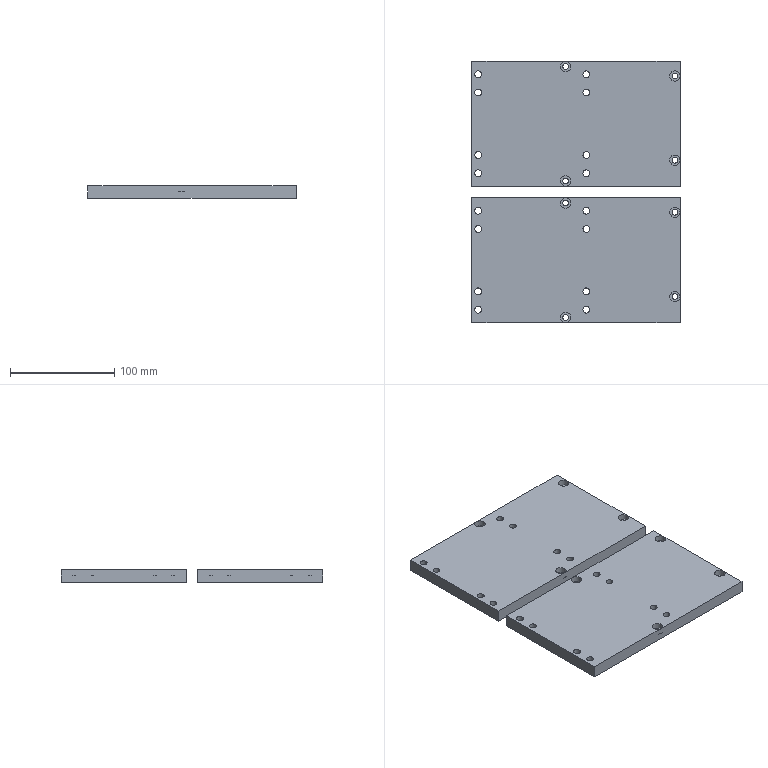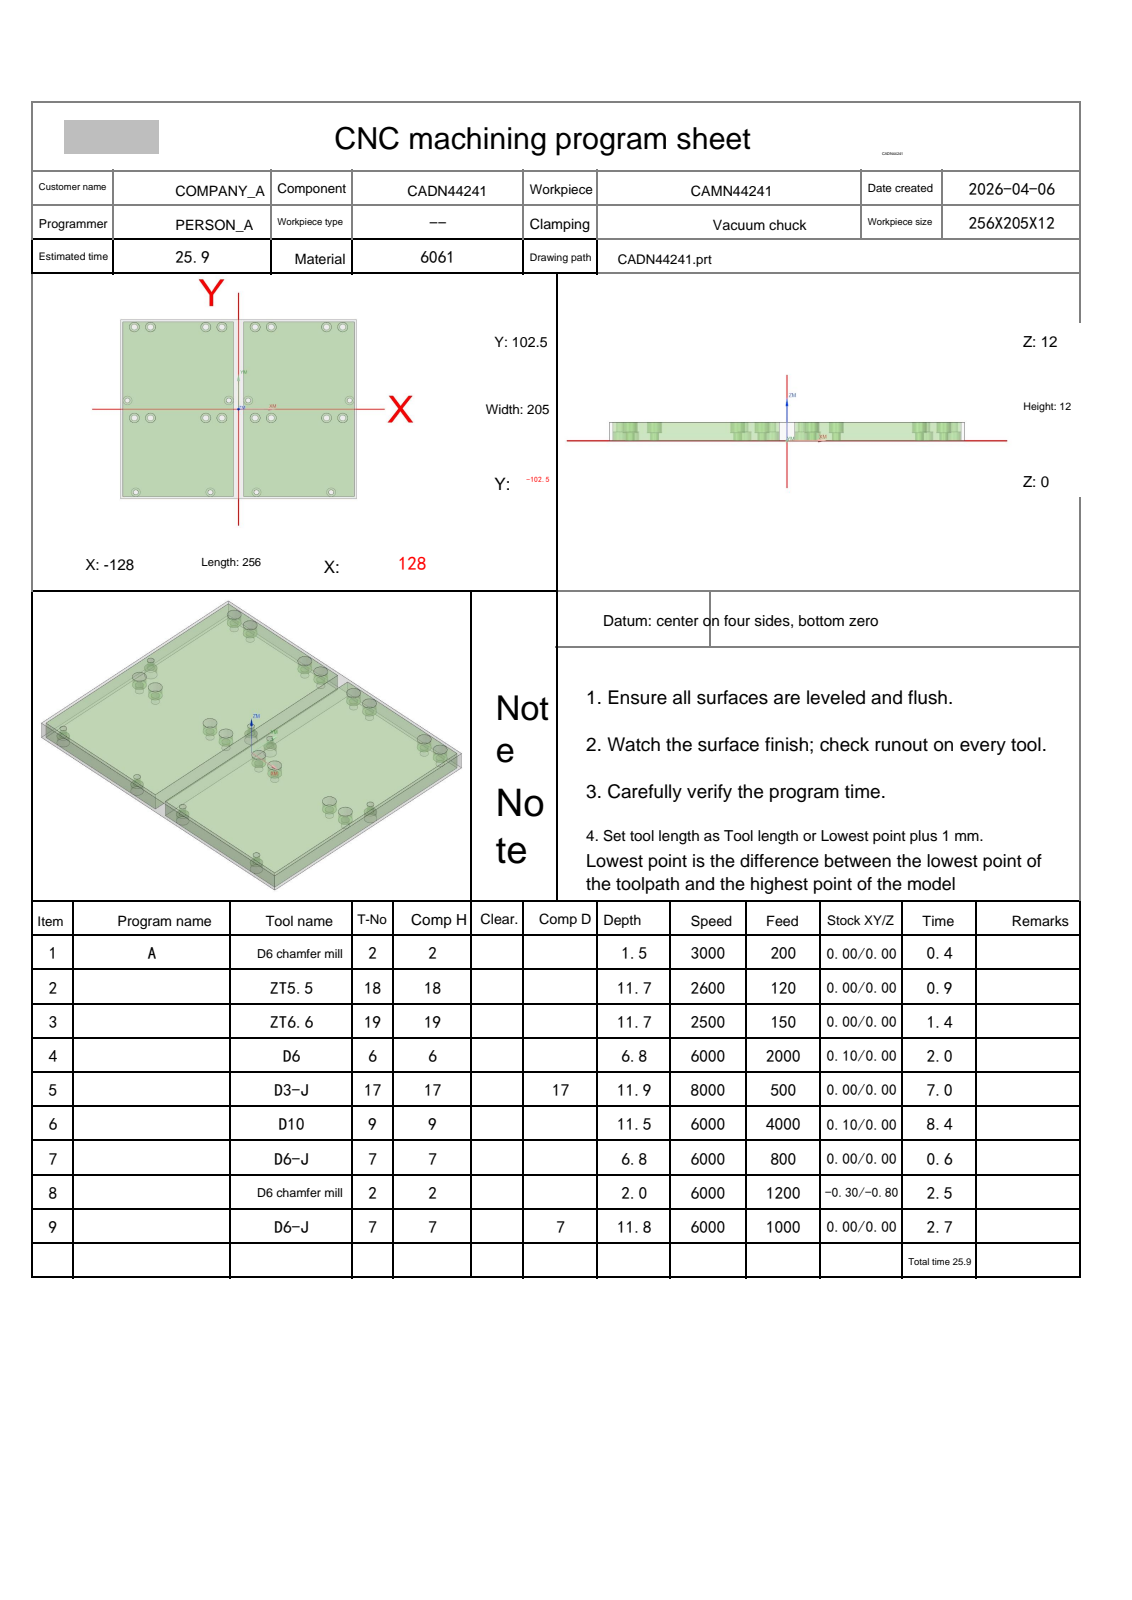NC program | NX | posted by the shop | part box 200 x 251 x 12 mm
Lines 1 to 557 of 3499:
%
O0001
(Machine time: 27.62 MIN)
(===Total Tool:7===)
(T2=D6 chamfer mill   D=6.   R=0.   D-  H02 Z=10.   )
(T18=ZT5.5  D=5.5  DR_a=118 D-  H18 Z=0.3   )
(T19=ZT6.6  D=6.6  DR_a=118 D-  H19 Z=0.3   )
(T6=D6      D=6.   R=0.   D-  H06 Z=5.2   )
(T17=D3-J   D=3.   R=0.   D17 H17 Z=0.15  )
(T9=D10     D=10.  R=0.   D-  H09 Z=0.5   )
(T7=D6-J    D=6.   R=0.   D-  H07 Z=0.2   )
G80 G90 G17 G49 G40
G91 G28 Z0
M01
N1 T02 M06
(D6 chamfer mill  D=6. R=0. H=02 ce=0.00 di=0.00)
G00 G90 G54 X100.5 Y-95. M03 S3000
G43 H02 Z32.
M08
G98 G81 X100.5 Y-95. Z10.5 R13. F200.
X19.5
X-30.5
X-111.5
X-113. Y-10.
X-120.5 Y10.
X-95.5 Y-10.
X-35.5
X-18.
X-10.5 Y10.
X10.5
X18. Y-10.
X35.5
X95.5
X113.
X120.5 Y10.
X113. Y94.
X95.5
X35.5
X18.
X-18.
X-35.5
X-95.5
X-113.
G80
G00 Z32.
G91 G28 Z0.0
M05
M09
G91 G28 Z0.0
M01
N2 T18 M06
(ZT5.5 D=5.5 DR_a=118 H=18)
G00 G90 G54 X10.5 Y10. M03 S2600
G43 H18 Z32.
M08
G98 G83 X10.5 Y10. Z.3 R13. F120. Q1.5
X-10.5
X-120.5
X-111.5 Y-95.
X-30.5
X19.5
X100.5
X120.5 Y10.
G80
G00 Z32.
G91 G28 Z0.0
M05
M09
G91 G28 Z0.0
M01
N3 T19 M06
(ZT6.6 D=6.6 DR_a=118 H=19)
G00 G90 G54 X-113. Y94. M03 S2500
G43 H19 Z32.
M08
G98 G83 X-113. Y94. Z.3 R13. F150. Q3.
X-95.5
X-35.5
X-18.
X18.
X35.5
X95.5
X113.
Y-10.
X95.5
X35.5
X18.
X-18.
X-35.5
X-95.5
X-113.
G80
G00 Z32.
G91 G28 Z0.0
M05
M09
G91 G28 Z0.0
M01
N4 T06 M06
(D6  D=6. R=0. H=06 ce=0.10 di=0.00)
G00 G90 G54 X18. Y94. M03 S6000
G43 H06 Z32.
M08
Z12.3
G03 X16.8 Y92.8 I0.0 J-1.2 F2000.
X18. Y91.6 I1.2 J0.0
X18. Y91.6 Z11.8 I0.0 J2.4
X18. Y91.6 Z11.3 I0.0 J2.4
X18. Y91.6 Z10.8 I0.0 J2.4
X18. Y91.6 Z10.3 I0.0 J2.4
X18. Y91.6 Z9.8 I0.0 J2.4
X18. Y91.6 Z9.3 I0.0 J2.4
X18. Y91.6 Z8.8 I0.0 J2.4
X18. Y91.6 Z8.3 I0.0 J2.4
X18. Y91.6 Z7.8 I0.0 J2.4
X18. Y91.6 Z7.3 I0.0 J2.4
X18. Y91.6 Z6.8 I0.0 J2.4
X18. Y91.6 Z6.3 I0.0 J2.4
X18. Y91.6 Z5.8 I0.0 J2.4
X18. Y91.6 Z5.3 I0.0 J2.4
X20.283 Y93.258 Z5.2 I0.0 J2.4
X20.4 Y94. I-2.283 J.742
X18. Y96.4 I-2.4 J0.0
X15.6 Y94. I0.0 J-2.4
X18. Y91.6 I2.4 J0.0
X20.283 Y93.258 I0.0 J2.4
X20.341 Y93.629 I-1.141 J.371
X19.141 Y94.829 I-1.2 J0.0
X18. Y94. I0.0 J-1.2
G00 Z32.
X35.5
Z12.3
G03 X34.3 Y92.8 I0.0 J-1.2
X35.5 Y91.6 I1.2 J0.0
X35.5 Y91.6 Z11.8 I0.0 J2.4
X35.5 Y91.6 Z11.3 I0.0 J2.4
X35.5 Y91.6 Z10.8 I0.0 J2.4
X35.5 Y91.6 Z10.3 I0.0 J2.4
X35.5 Y91.6 Z9.8 I0.0 J2.4
X35.5 Y91.6 Z9.3 I0.0 J2.4
X35.5 Y91.6 Z8.8 I0.0 J2.4
X35.5 Y91.6 Z8.3 I0.0 J2.4
X35.5 Y91.6 Z7.8 I0.0 J2.4
X35.5 Y91.6 Z7.3 I0.0 J2.4
X35.5 Y91.6 Z6.8 I0.0 J2.4
X35.5 Y91.6 Z6.3 I0.0 J2.4
X35.5 Y91.6 Z5.8 I0.0 J2.4
X35.5 Y91.6 Z5.3 I0.0 J2.4
X37.783 Y93.258 Z5.2 I0.0 J2.4
X37.9 Y94. I-2.283 J.742
X35.5 Y96.4 I-2.4 J0.0
X33.1 Y94. I0.0 J-2.4
X35.5 Y91.6 I2.4 J0.0
X37.783 Y93.258 I0.0 J2.4
X37.841 Y93.629 I-1.141 J.371
X36.641 Y94.829 I-1.2 J0.0
X35.5 Y94. I0.0 J-1.2
G00 Z32.
X-18.
Z12.3
G03 X-19.2 Y92.8 I0.0 J-1.2
X-18. Y91.6 I1.2 J0.0
X-18. Y91.6 Z11.8 I0.0 J2.4
X-18. Y91.6 Z11.3 I0.0 J2.4
X-18. Y91.6 Z10.8 I0.0 J2.4
X-18. Y91.6 Z10.3 I0.0 J2.4
X-18. Y91.6 Z9.8 I0.0 J2.4
X-18. Y91.6 Z9.3 I0.0 J2.4
X-18. Y91.6 Z8.8 I0.0 J2.4
X-18. Y91.6 Z8.3 I0.0 J2.4
X-18. Y91.6 Z7.8 I0.0 J2.4
X-18. Y91.6 Z7.3 I0.0 J2.4
X-18. Y91.6 Z6.8 I0.0 J2.4
X-18. Y91.6 Z6.3 I0.0 J2.4
X-18. Y91.6 Z5.8 I0.0 J2.4
X-18. Y91.6 Z5.3 I0.0 J2.4
X-15.717 Y93.258 Z5.2 I0.0 J2.4
X-15.6 Y94. I-2.283 J.742
X-18. Y96.4 I-2.4 J0.0
X-20.4 Y94. I0.0 J-2.4
X-18. Y91.6 I2.4 J0.0
X-15.717 Y93.258 I0.0 J2.4
X-15.659 Y93.629 I-1.141 J.371
X-16.859 Y94.829 I-1.2 J0.0
X-18. Y94. I0.0 J-1.2
G00 Z32.
X-35.5
Z12.3
G03 X-36.7 Y92.8 I0.0 J-1.2
X-35.5 Y91.6 I1.2 J0.0
X-35.5 Y91.6 Z11.8 I0.0 J2.4
X-35.5 Y91.6 Z11.3 I0.0 J2.4
X-35.5 Y91.6 Z10.8 I0.0 J2.4
X-35.5 Y91.6 Z10.3 I0.0 J2.4
X-35.5 Y91.6 Z9.8 I0.0 J2.4
X-35.5 Y91.6 Z9.3 I0.0 J2.4
X-35.5 Y91.6 Z8.8 I0.0 J2.4
X-35.5 Y91.6 Z8.3 I0.0 J2.4
X-35.5 Y91.6 Z7.8 I0.0 J2.4
X-35.5 Y91.6 Z7.3 I0.0 J2.4
X-35.5 Y91.6 Z6.8 I0.0 J2.4
X-35.5 Y91.6 Z6.3 I0.0 J2.4
X-35.5 Y91.6 Z5.8 I0.0 J2.4
X-35.5 Y91.6 Z5.3 I0.0 J2.4
X-33.217 Y93.258 Z5.2 I0.0 J2.4
X-33.1 Y94. I-2.283 J.742
X-35.5 Y96.4 I-2.4 J0.0
X-37.9 Y94. I0.0 J-2.4
X-35.5 Y91.6 I2.4 J0.0
X-33.217 Y93.258 I0.0 J2.4
X-33.159 Y93.629 I-1.141 J.371
X-34.359 Y94.829 I-1.2 J0.0
X-35.5 Y94. I0.0 J-1.2
G00 Z32.
X-95.5
Z12.3
G03 X-96.7 Y92.8 I0.0 J-1.2
X-95.5 Y91.6 I1.2 J0.0
X-95.5 Y91.6 Z11.8 I0.0 J2.4
X-95.5 Y91.6 Z11.3 I0.0 J2.4
X-95.5 Y91.6 Z10.8 I0.0 J2.4
X-95.5 Y91.6 Z10.3 I0.0 J2.4
X-95.5 Y91.6 Z9.8 I0.0 J2.4
X-95.5 Y91.6 Z9.3 I0.0 J2.4
X-95.5 Y91.6 Z8.8 I0.0 J2.4
X-95.5 Y91.6 Z8.3 I0.0 J2.4
X-95.5 Y91.6 Z7.8 I0.0 J2.4
X-95.5 Y91.6 Z7.3 I0.0 J2.4
X-95.5 Y91.6 Z6.8 I0.0 J2.4
X-95.5 Y91.6 Z6.3 I0.0 J2.4
X-95.5 Y91.6 Z5.8 I0.0 J2.4
X-95.5 Y91.6 Z5.3 I0.0 J2.4
X-93.217 Y93.258 Z5.2 I0.0 J2.4
X-93.1 Y94. I-2.283 J.742
X-95.5 Y96.4 I-2.4 J0.0
X-97.9 Y94. I0.0 J-2.4
X-95.5 Y91.6 I2.4 J0.0
X-93.217 Y93.258 I0.0 J2.4
X-93.159 Y93.629 I-1.141 J.371
X-94.359 Y94.829 I-1.2 J0.0
X-95.5 Y94. I0.0 J-1.2
G00 Z32.
X-113.
Z12.3
G03 X-114.2 Y92.8 I0.0 J-1.2
X-113. Y91.6 I1.2 J0.0
X-113. Y91.6 Z11.8 I0.0 J2.4
X-113. Y91.6 Z11.3 I0.0 J2.4
X-113. Y91.6 Z10.8 I0.0 J2.4
X-113. Y91.6 Z10.3 I0.0 J2.4
X-113. Y91.6 Z9.8 I0.0 J2.4
X-113. Y91.6 Z9.3 I0.0 J2.4
X-113. Y91.6 Z8.8 I0.0 J2.4
X-113. Y91.6 Z8.3 I0.0 J2.4
X-113. Y91.6 Z7.8 I0.0 J2.4
X-113. Y91.6 Z7.3 I0.0 J2.4
X-113. Y91.6 Z6.8 I0.0 J2.4
X-113. Y91.6 Z6.3 I0.0 J2.4
X-113. Y91.6 Z5.8 I0.0 J2.4
X-113. Y91.6 Z5.3 I0.0 J2.4
X-110.717 Y93.258 Z5.2 I0.0 J2.4
X-110.6 Y94. I-2.283 J.742
X-113. Y96.4 I-2.4 J0.0
X-115.4 Y94. I0.0 J-2.4
X-113. Y91.6 I2.4 J0.0
X-110.717 Y93.258 I0.0 J2.4
X-110.659 Y93.629 I-1.141 J.371
X-111.859 Y94.829 I-1.2 J0.0
X-113. Y94. I0.0 J-1.2
G00 Z32.
Y-10.
Z12.3
G03 X-114.2 Y-11.2 I0.0 J-1.2
X-113. Y-12.4 I1.2 J0.0
X-113. Y-12.4 Z11.8 I0.0 J2.4
X-113. Y-12.4 Z11.3 I0.0 J2.4
X-113. Y-12.4 Z10.8 I0.0 J2.4
X-113. Y-12.4 Z10.3 I0.0 J2.4
X-113. Y-12.4 Z9.8 I0.0 J2.4
X-113. Y-12.4 Z9.3 I0.0 J2.4
X-113. Y-12.4 Z8.8 I0.0 J2.4
X-113. Y-12.4 Z8.3 I0.0 J2.4
X-113. Y-12.4 Z7.8 I0.0 J2.4
X-113. Y-12.4 Z7.3 I0.0 J2.4
X-113. Y-12.4 Z6.8 I0.0 J2.4
X-113. Y-12.4 Z6.3 I0.0 J2.4
X-113. Y-12.4 Z5.8 I0.0 J2.4
X-113. Y-12.4 Z5.3 I0.0 J2.4
X-110.717 Y-10.742 Z5.2 I0.0 J2.4
X-110.6 Y-10. I-2.283 J.742
X-113. Y-7.6 I-2.4 J0.0
X-115.4 Y-10. I0.0 J-2.4
X-113. Y-12.4 I2.4 J0.0
X-110.717 Y-10.742 I0.0 J2.4
X-110.659 Y-10.371 I-1.141 J.371
X-111.859 Y-9.171 I-1.2 J0.0
X-113. Y-10. I0.0 J-1.2
G00 Z32.
X-95.5
Z12.3
G03 X-96.7 Y-11.2 I0.0 J-1.2
X-95.5 Y-12.4 I1.2 J0.0
X-95.5 Y-12.4 Z11.8 I0.0 J2.4
X-95.5 Y-12.4 Z11.3 I0.0 J2.4
X-95.5 Y-12.4 Z10.8 I0.0 J2.4
X-95.5 Y-12.4 Z10.3 I0.0 J2.4
X-95.5 Y-12.4 Z9.8 I0.0 J2.4
X-95.5 Y-12.4 Z9.3 I0.0 J2.4
X-95.5 Y-12.4 Z8.8 I0.0 J2.4
X-95.5 Y-12.4 Z8.3 I0.0 J2.4
X-95.5 Y-12.4 Z7.8 I0.0 J2.4
X-95.5 Y-12.4 Z7.3 I0.0 J2.4
X-95.5 Y-12.4 Z6.8 I0.0 J2.4
X-95.5 Y-12.4 Z6.3 I0.0 J2.4
X-95.5 Y-12.4 Z5.8 I0.0 J2.4
X-95.5 Y-12.4 Z5.3 I0.0 J2.4
X-93.217 Y-10.742 Z5.2 I0.0 J2.4
X-93.1 Y-10. I-2.283 J.742
X-95.5 Y-7.6 I-2.4 J0.0
X-97.9 Y-10. I0.0 J-2.4
X-95.5 Y-12.4 I2.4 J0.0
X-93.217 Y-10.742 I0.0 J2.4
X-93.159 Y-10.371 I-1.141 J.371
X-94.359 Y-9.171 I-1.2 J0.0
X-95.5 Y-10. I0.0 J-1.2
G00 Z32.
X-35.5
Z12.3
G03 X-36.7 Y-11.2 I0.0 J-1.2
X-35.5 Y-12.4 I1.2 J0.0
X-35.5 Y-12.4 Z11.8 I0.0 J2.4
X-35.5 Y-12.4 Z11.3 I0.0 J2.4
X-35.5 Y-12.4 Z10.8 I0.0 J2.4
X-35.5 Y-12.4 Z10.3 I0.0 J2.4
X-35.5 Y-12.4 Z9.8 I0.0 J2.4
X-35.5 Y-12.4 Z9.3 I0.0 J2.4
X-35.5 Y-12.4 Z8.8 I0.0 J2.4
X-35.5 Y-12.4 Z8.3 I0.0 J2.4
X-35.5 Y-12.4 Z7.8 I0.0 J2.4
X-35.5 Y-12.4 Z7.3 I0.0 J2.4
X-35.5 Y-12.4 Z6.8 I0.0 J2.4
X-35.5 Y-12.4 Z6.3 I0.0 J2.4
X-35.5 Y-12.4 Z5.8 I0.0 J2.4
X-35.5 Y-12.4 Z5.3 I0.0 J2.4
X-33.217 Y-10.742 Z5.2 I0.0 J2.4
X-33.1 Y-10. I-2.283 J.742
X-35.5 Y-7.6 I-2.4 J0.0
X-37.9 Y-10. I0.0 J-2.4
X-35.5 Y-12.4 I2.4 J0.0
X-33.217 Y-10.742 I0.0 J2.4
X-33.159 Y-10.371 I-1.141 J.371
X-34.359 Y-9.171 I-1.2 J0.0
X-35.5 Y-10. I0.0 J-1.2
G00 Z32.
X-18.
Z12.3
G03 X-19.2 Y-11.2 I0.0 J-1.2
X-18. Y-12.4 I1.2 J0.0
X-18. Y-12.4 Z11.8 I0.0 J2.4
X-18. Y-12.4 Z11.3 I0.0 J2.4
X-18. Y-12.4 Z10.8 I0.0 J2.4
X-18. Y-12.4 Z10.3 I0.0 J2.4
X-18. Y-12.4 Z9.8 I0.0 J2.4
X-18. Y-12.4 Z9.3 I0.0 J2.4
X-18. Y-12.4 Z8.8 I0.0 J2.4
X-18. Y-12.4 Z8.3 I0.0 J2.4
X-18. Y-12.4 Z7.8 I0.0 J2.4
X-18. Y-12.4 Z7.3 I0.0 J2.4
X-18. Y-12.4 Z6.8 I0.0 J2.4
X-18. Y-12.4 Z6.3 I0.0 J2.4
X-18. Y-12.4 Z5.8 I0.0 J2.4
X-18. Y-12.4 Z5.3 I0.0 J2.4
X-15.717 Y-10.742 Z5.2 I0.0 J2.4
X-15.6 Y-10. I-2.283 J.742
X-18. Y-7.6 I-2.4 J0.0
X-20.4 Y-10. I0.0 J-2.4
X-18. Y-12.4 I2.4 J0.0
X-15.717 Y-10.742 I0.0 J2.4
X-15.659 Y-10.371 I-1.141 J.371
X-16.859 Y-9.171 I-1.2 J0.0
X-18. Y-10. I0.0 J-1.2
G00 Z32.
X18.
Z12.3
G03 X16.8 Y-11.2 I0.0 J-1.2
X18. Y-12.4 I1.2 J0.0
X18. Y-12.4 Z11.8 I0.0 J2.4
X18. Y-12.4 Z11.3 I0.0 J2.4
X18. Y-12.4 Z10.8 I0.0 J2.4
X18. Y-12.4 Z10.3 I0.0 J2.4
X18. Y-12.4 Z9.8 I0.0 J2.4
X18. Y-12.4 Z9.3 I0.0 J2.4
X18. Y-12.4 Z8.8 I0.0 J2.4
X18. Y-12.4 Z8.3 I0.0 J2.4
X18. Y-12.4 Z7.8 I0.0 J2.4
X18. Y-12.4 Z7.3 I0.0 J2.4
X18. Y-12.4 Z6.8 I0.0 J2.4
X18. Y-12.4 Z6.3 I0.0 J2.4
X18. Y-12.4 Z5.8 I0.0 J2.4
X18. Y-12.4 Z5.3 I0.0 J2.4
X20.283 Y-10.742 Z5.2 I0.0 J2.4
X20.4 Y-10. I-2.283 J.742
X18. Y-7.6 I-2.4 J0.0
X15.6 Y-10. I0.0 J-2.4
X18. Y-12.4 I2.4 J0.0
X20.283 Y-10.742 I0.0 J2.4
X20.341 Y-10.371 I-1.141 J.371
X19.141 Y-9.171 I-1.2 J0.0
X18. Y-10. I0.0 J-1.2
G00 Z32.
X35.5
Z12.3
G03 X34.3 Y-11.2 I0.0 J-1.2
X35.5 Y-12.4 I1.2 J0.0
X35.5 Y-12.4 Z11.8 I0.0 J2.4
X35.5 Y-12.4 Z11.3 I0.0 J2.4
X35.5 Y-12.4 Z10.8 I0.0 J2.4
X35.5 Y-12.4 Z10.3 I0.0 J2.4
X35.5 Y-12.4 Z9.8 I0.0 J2.4
X35.5 Y-12.4 Z9.3 I0.0 J2.4
X35.5 Y-12.4 Z8.8 I0.0 J2.4
X35.5 Y-12.4 Z8.3 I0.0 J2.4
X35.5 Y-12.4 Z7.8 I0.0 J2.4
X35.5 Y-12.4 Z7.3 I0.0 J2.4
X35.5 Y-12.4 Z6.8 I0.0 J2.4
X35.5 Y-12.4 Z6.3 I0.0 J2.4
X35.5 Y-12.4 Z5.8 I0.0 J2.4
X35.5 Y-12.4 Z5.3 I0.0 J2.4
X37.783 Y-10.742 Z5.2 I0.0 J2.4
X37.9 Y-10. I-2.283 J.742
X35.5 Y-7.6 I-2.4 J0.0
X33.1 Y-10. I0.0 J-2.4
X35.5 Y-12.4 I2.4 J0.0
X37.783 Y-10.742 I0.0 J2.4
X37.841 Y-10.371 I-1.141 J.371
X36.641 Y-9.171 I-1.2 J0.0
X35.5 Y-10. I0.0 J-1.2
G00 Z32.
X95.5
Z12.3
G03 X94.3 Y-11.2 I0.0 J-1.2
X95.5 Y-12.4 I1.2 J0.0
X95.5 Y-12.4 Z11.8 I0.0 J2.4
X95.5 Y-12.4 Z11.3 I0.0 J2.4
X95.5 Y-12.4 Z10.8 I0.0 J2.4
X95.5 Y-12.4 Z10.3 I0.0 J2.4
X95.5 Y-12.4 Z9.8 I0.0 J2.4
X95.5 Y-12.4 Z9.3 I0.0 J2.4
X95.5 Y-12.4 Z8.8 I0.0 J2.4
X95.5 Y-12.4 Z8.3 I0.0 J2.4
X95.5 Y-12.4 Z7.8 I0.0 J2.4
X95.5 Y-12.4 Z7.3 I0.0 J2.4
X95.5 Y-12.4 Z6.8 I0.0 J2.4
X95.5 Y-12.4 Z6.3 I0.0 J2.4
X95.5 Y-12.4 Z5.8 I0.0 J2.4
X95.5 Y-12.4 Z5.3 I0.0 J2.4
X97.783 Y-10.742 Z5.2 I0.0 J2.4
X97.9 Y-10. I-2.283 J.742
X95.5 Y-7.6 I-2.4 J0.0
X93.1 Y-10. I0.0 J-2.4
X95.5 Y-12.4 I2.4 J0.0
X97.783 Y-10.742 I0.0 J2.4
X97.841 Y-10.371 I-1.141 J.371
X96.641 Y-9.171 I-1.2 J0.0
X95.5 Y-10. I0.0 J-1.2
G00 Z32.
X113.
Z12.3
G03 X111.8 Y-11.2 I0.0 J-1.2
X113. Y-12.4 I1.2 J0.0
X113. Y-12.4 Z11.8 I0.0 J2.4
X113. Y-12.4 Z11.3 I0.0 J2.4
X113. Y-12.4 Z10.8 I0.0 J2.4
X113. Y-12.4 Z10.3 I0.0 J2.4
X113. Y-12.4 Z9.8 I0.0 J2.4
X113. Y-12.4 Z9.3 I0.0 J2.4
X113. Y-12.4 Z8.8 I0.0 J2.4
X113. Y-12.4 Z8.3 I0.0 J2.4
X113. Y-12.4 Z7.8 I0.0 J2.4
X113. Y-12.4 Z7.3 I0.0 J2.4
X113. Y-12.4 Z6.8 I0.0 J2.4
X113. Y-12.4 Z6.3 I0.0 J2.4
X113. Y-12.4 Z5.8 I0.0 J2.4
X113. Y-12.4 Z5.3 I0.0 J2.4
X115.283 Y-10.742 Z5.2 I0.0 J2.4
X115.4 Y-10. I-2.283 J.742
X113. Y-7.6 I-2.4 J0.0
X110.6 Y-10. I0.0 J-2.4
X113. Y-12.4 I2.4 J0.0
X115.283 Y-10.742 I0.0 J2.4
X115.341 Y-10.371 I-1.141 J.371
X114.141 Y-9.171 I-1.2 J0.0
X113. Y-10. I0.0 J-1.2
G00 Z32.
Y94.
Z12.3
G03 X111.8 Y92.8 I0.0 J-1.2
X113. Y91.6 I1.2 J0.0
X113. Y91.6 Z11.8 I0.0 J2.4
X113. Y91.6 Z11.3 I0.0 J2.4
X113. Y91.6 Z10.8 I0.0 J2.4
X113. Y91.6 Z10.3 I0.0 J2.4
X113. Y91.6 Z9.8 I0.0 J2.4
X113. Y91.6 Z9.3 I0.0 J2.4
X113. Y91.6 Z8.8 I0.0 J2.4
X113. Y91.6 Z8.3 I0.0 J2.4
X113. Y91.6 Z7.8 I0.0 J2.4
X113. Y91.6 Z7.3 I0.0 J2.4
X113. Y91.6 Z6.8 I0.0 J2.4
X113. Y91.6 Z6.3 I0.0 J2.4
X113. Y91.6 Z5.8 I0.0 J2.4
X113. Y91.6 Z5.3 I0.0 J2.4
X115.283 Y93.258 Z5.2 I0.0 J2.4
X115.4 Y94. I-2.283 J.742
X113. Y96.4 I-2.4 J0.0
X110.6 Y94. I0.0 J-2.4
X113. Y91.6 I2.4 J0.0
X115.283 Y93.258 I0.0 J2.4
X115.341 Y93.629 I-1.141 J.371
X114.141 Y94.829 I-1.2 J0.0
X113. Y94. I0.0 J-1.2
G00 Z32.
X95.5
Z12.3
G03 X94.3 Y92.8 I0.0 J-1.2
X95.5 Y91.6 I1.2 J0.0
X95.5 Y91.6 Z11.8 I0.0 J2.4
X95.5 Y91.6 Z11.3 I0.0 J2.4
X95.5 Y91.6 Z10.8 I0.0 J2.4
X95.5 Y91.6 Z10.3 I0.0 J2.4
X95.5 Y91.6 Z9.8 I0.0 J2.4
X95.5 Y91.6 Z9.3 I0.0 J2.4
X95.5 Y91.6 Z8.8 I0.0 J2.4
X95.5 Y91.6 Z8.3 I0.0 J2.4
X95.5 Y91.6 Z7.8 I0.0 J2.4
X95.5 Y91.6 Z7.3 I0.0 J2.4
X95.5 Y91.6 Z6.8 I0.0 J2.4
X95.5 Y91.6 Z6.3 I0.0 J2.4
X95.5 Y91.6 Z5.8 I0.0 J2.4
X95.5 Y91.6 Z5.3 I0.0 J2.4
X97.783 Y93.258 Z5.2 I0.0 J2.4
X97.9 Y94. I-2.283 J.742
X95.5 Y96.4 I-2.4 J0.0
X93.1 Y94. I0.0 J-2.4
X95.5 Y91.6 I2.4 J0.0
X97.783 Y93.258 I0.0 J2.4
X97.841 Y93.629 I-1.141 J.371
X96.641 Y94.829 I-1.2 J0.0
X95.5 Y94. I0.0 J-1.2
G00 Z32.
G91 G28 Z0.0
M05
M09
G91 G28 Z0.0
M01